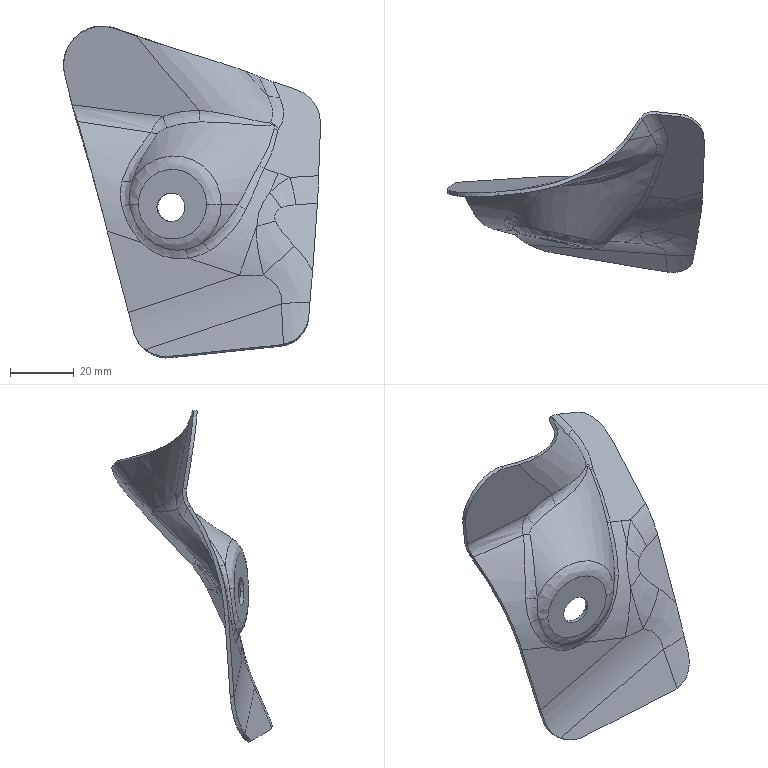Part | 1 solid | 100 faces | box 80.756 x 50.37 x 104.302 mm | volume 8588 mm3 | spline 79 | plane 10 | cylinder 10 | other 1 | commonest cylinder face diameters 9 x2 100 x2 102.4 x2 60 x1 62.4 x1 72.4 x1